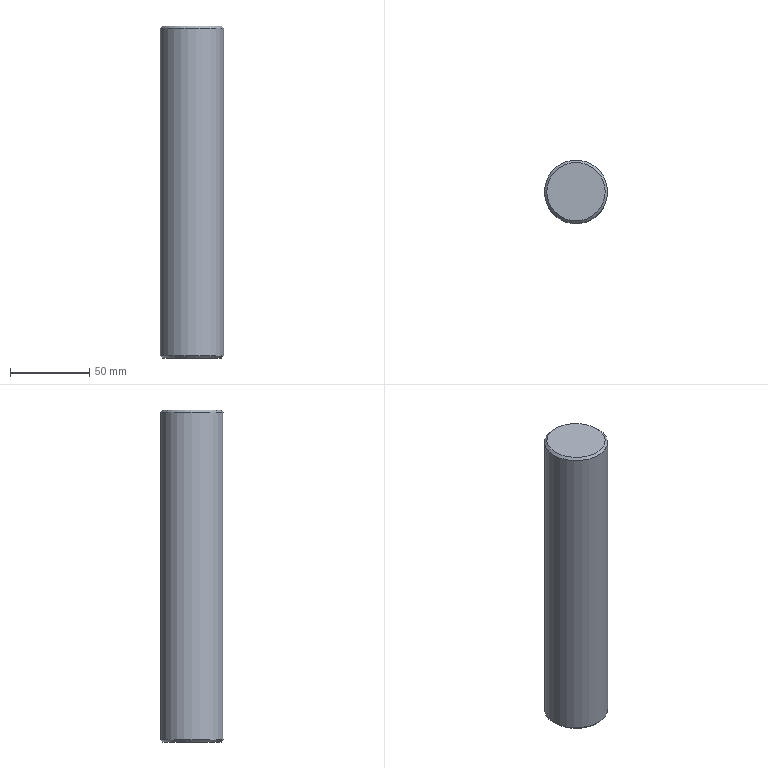Part | STEP file | 车灯-后视镜_id18_x_t | 1 solid | 9 faces | box 40 x 40 x 210 mm | volume 261823 mm3 | cylinder 3 | plane 3 | cone 3 | commonest cylinder face diameters 8.6 x1 10 x1 40 x1
STEP:
#1=CARTESIAN_POINT('',(35.,50.,-162.));
#2=VERTEX_POINT('',#1);
#3=CARTESIAN_POINT('',(15.,50.,-162.));
#4=DIRECTION('',(0.,0.,-1.));
#5=DIRECTION('',(1.,0.,0.));
#6=AXIS2_PLACEMENT_3D('',#3,#4,#5);
#7=CIRCLE('',#6,20.);
#8=EDGE_CURVE('',#2,#2,#7,.T.);
#9=ORIENTED_EDGE('',*,*,#8,.T.);
#10=EDGE_LOOP('',(#9));
#11=FACE_BOUND('',#10,.T.);
#12=CARTESIAN_POINT('',(-5.,50.,-369.));
#13=VERTEX_POINT('',#12);
#14=CARTESIAN_POINT('',(15.,50.,-369.));
#15=DIRECTION('',(0.,0.,1.));
#16=DIRECTION('',(-1.,0.,0.));
#17=AXIS2_PLACEMENT_3D('',#14,#15,#16);
#18=CIRCLE('',#17,20.);
#19=EDGE_CURVE('',#13,#13,#18,.T.);
#20=ORIENTED_EDGE('',*,*,#19,.T.);
#21=EDGE_LOOP('',(#20));
#22=FACE_BOUND('',#21,.T.);
#23=CARTESIAN_POINT('',(15.,50.,-330.5));
#24=DIRECTION('',(0.,0.,1.));
#25=DIRECTION('',(-1.,0.,0.));
#26=AXIS2_PLACEMENT_3D('',#23,#24,#25);
#27=CYLINDRICAL_SURFACE('',#26,20.);
#28=ADVANCED_FACE('',(#11,#22),#27,.T.);
#29=CARTESIAN_POINT('',(33.5,50.,-160.5));
#30=VERTEX_POINT('',#29);
#31=CARTESIAN_POINT('',(15.,50.,-160.5));
#32=DIRECTION('',(0.,0.,1.));
#33=DIRECTION('',(1.,0.,0.));
#34=AXIS2_PLACEMENT_3D('',#31,#32,#33);
#35=CIRCLE('',#34,18.5);
#36=EDGE_CURVE('',#30,#30,#35,.T.);
#37=ORIENTED_EDGE('',*,*,#36,.T.);
#38=EDGE_LOOP('',(#37));
#39=FACE_OUTER_BOUND('',#38,.T.);
#40=CARTESIAN_POINT('',(15.,50.,-160.5));
#41=DIRECTION('',(0.,0.,1.));
#42=DIRECTION('',(-1.,0.,0.));
#43=AXIS2_PLACEMENT_3D('',#40,#41,#42);
#44=PLANE('',#43);
#45=ADVANCED_FACE('',(#39),#44,.T.);
#46=CARTESIAN_POINT('',(-3.5,50.,-370.5));
#47=VERTEX_POINT('',#46);
#48=CARTESIAN_POINT('',(15.,50.,-370.5));
#49=DIRECTION('',(0.,0.,-1.));
#50=DIRECTION('',(-1.,0.,0.));
#51=AXIS2_PLACEMENT_3D('',#48,#49,#50);
#52=CIRCLE('',#51,18.5);
#53=EDGE_CURVE('',#47,#47,#52,.T.);
#54=ORIENTED_EDGE('',*,*,#53,.T.);
#55=EDGE_LOOP('',(#54));
#56=FACE_BOUND('',#55,.T.);
#57=CARTESIAN_POINT('',(10.,50.,-370.5));
#58=VERTEX_POINT('',#57);
#59=CARTESIAN_POINT('',(15.,50.,-370.5));
#60=DIRECTION('',(0.,0.,-1.));
#61=DIRECTION('',(-1.,0.,0.));
#62=AXIS2_PLACEMENT_3D('',#59,#60,#61);
#63=CIRCLE('',#62,5.);
#64=EDGE_CURVE('',#58,#58,#63,.T.);
#65=ORIENTED_EDGE('',*,*,#64,.F.);
#66=EDGE_LOOP('',(#65));
#67=FACE_BOUND('',#66,.T.);
#68=CARTESIAN_POINT('',(15.,50.,-370.5));
#69=DIRECTION('',(0.,0.,-1.));
#70=DIRECTION('',(1.,0.,0.));
#71=AXIS2_PLACEMENT_3D('',#68,#69,#70);
#72=PLANE('',#71);
#73=ADVANCED_FACE('',(#56,#67),#72,.T.);
#74=CARTESIAN_POINT('',(19.3,50.,-347.5));
#75=VERTEX_POINT('',#74);
#76=CARTESIAN_POINT('',(15.,50.,-347.5));
#77=DIRECTION('',(0.,0.,1.));
#78=DIRECTION('',(1.,0.,0.));
#79=AXIS2_PLACEMENT_3D('',#76,#77,#78);
#80=CIRCLE('',#79,4.3);
#81=EDGE_CURVE('',#75,#75,#80,.T.);
#82=ORIENTED_EDGE('',*,*,#81,.T.);
#83=EDGE_LOOP('',(#82));
#84=FACE_BOUND('',#83,.T.);
#85=CARTESIAN_POINT('',(10.7,50.,-350.5));
#86=VERTEX_POINT('',#85);
#87=CARTESIAN_POINT('',(15.,50.,-350.5));
#88=DIRECTION('',(0.,0.,1.));
#89=DIRECTION('',(-1.,0.,0.));
#90=AXIS2_PLACEMENT_3D('',#87,#88,#89);
#91=CIRCLE('',#90,4.3);
#92=EDGE_CURVE('',#86,#86,#91,.T.);
#93=ORIENTED_EDGE('',*,*,#92,.F.);
#94=EDGE_LOOP('',(#93));
#95=FACE_BOUND('',#94,.T.);
#96=CARTESIAN_POINT('',(15.,50.,-350.5));
#97=DIRECTION('',(0.,0.,1.));
#98=DIRECTION('',(-1.,0.,0.));
#99=AXIS2_PLACEMENT_3D('',#96,#97,#98);
#100=CYLINDRICAL_SURFACE('',#99,4.3);
#101=ADVANCED_FACE('',(#84,#95),#100,.F.);
#102=ORIENTED_EDGE('',*,*,#81,.F.);
#103=EDGE_LOOP('',(#102));
#104=FACE_BOUND('',#103,.T.);
#105=CARTESIAN_POINT('',(15.,50.,-344.916));
#106=VERTEX_POINT('',#105);
#107=VERTEX_LOOP('',#106);
#108=FACE_BOUND('',#107,.T.);
#109=CARTESIAN_POINT('',(15.,50.,-344.916));
#110=DIRECTION('',(0.,0.,-1.));
#111=DIRECTION('',(1.,0.,0.));
#112=AXIS2_PLACEMENT_3D('',#109,#110,#111);
#113=CONICAL_SURFACE('',#112,0.,59.);
#114=ADVANCED_FACE('',(#104,#108),#113,.F.);
#115=ORIENTED_EDGE('',*,*,#92,.T.);
#116=EDGE_LOOP('',(#115));
#117=FACE_BOUND('',#116,.T.);
#118=CARTESIAN_POINT('',(20.,50.,-350.5));
#119=VERTEX_POINT('',#118);
#120=CARTESIAN_POINT('',(15.,50.,-350.5));
#121=DIRECTION('',(0.,0.,1.));
#122=DIRECTION('',(1.,0.,0.));
#123=AXIS2_PLACEMENT_3D('',#120,#121,#122);
#124=CIRCLE('',#123,5.);
#125=EDGE_CURVE('',#119,#119,#124,.T.);
#126=ORIENTED_EDGE('',*,*,#125,.F.);
#127=EDGE_LOOP('',(#126));
#128=FACE_BOUND('',#127,.T.);
#129=CARTESIAN_POINT('',(15.,50.,-350.5));
#130=DIRECTION('',(0.,0.,1.));
#131=DIRECTION('',(-1.,0.,0.));
#132=AXIS2_PLACEMENT_3D('',#129,#130,#131);
#133=PLANE('',#132);
#134=ADVANCED_FACE('',(#117,#128),#133,.F.);
#135=ORIENTED_EDGE('',*,*,#125,.T.);
#136=EDGE_LOOP('',(#135));
#137=FACE_BOUND('',#136,.T.);
#138=ORIENTED_EDGE('',*,*,#64,.T.);
#139=EDGE_LOOP('',(#138));
#140=FACE_BOUND('',#139,.T.);
#141=CARTESIAN_POINT('',(15.,50.,-370.5));
#142=DIRECTION('',(0.,0.,1.));
#143=DIRECTION('',(-1.,0.,0.));
#144=AXIS2_PLACEMENT_3D('',#141,#142,#143);
#145=CYLINDRICAL_SURFACE('',#144,5.);
#146=ADVANCED_FACE('',(#137,#140),#145,.F.);
#147=ORIENTED_EDGE('',*,*,#8,.F.);
#148=EDGE_LOOP('',(#147));
#149=FACE_BOUND('',#148,.T.);
#150=ORIENTED_EDGE('',*,*,#36,.F.);
#151=EDGE_LOOP('',(#150));
#152=FACE_BOUND('',#151,.T.);
#153=CARTESIAN_POINT('',(15.,50.,-160.5));
#154=DIRECTION('',(0.,0.,-1.));
#155=DIRECTION('',(-1.,0.,0.));
#156=AXIS2_PLACEMENT_3D('',#153,#154,#155);
#157=CONICAL_SURFACE('',#156,18.5,45.);
#158=ADVANCED_FACE('',(#149,#152),#157,.T.);
#159=ORIENTED_EDGE('',*,*,#53,.F.);
#160=EDGE_LOOP('',(#159));
#161=FACE_BOUND('',#160,.T.);
#162=ORIENTED_EDGE('',*,*,#19,.F.);
#163=EDGE_LOOP('',(#162));
#164=FACE_BOUND('',#163,.T.);
#165=CARTESIAN_POINT('',(15.,50.,-369.));
#166=DIRECTION('',(0.,0.,1.));
#167=DIRECTION('',(1.,0.,0.));
#168=AXIS2_PLACEMENT_3D('',#165,#166,#167);
#169=CONICAL_SURFACE('',#168,20.,45.);
#170=ADVANCED_FACE('',(#161,#164),#169,.T.);
#171=CLOSED_SHELL('',(#28,#45,#73,#101,#114,#134,#146,#158,#170));
#172=MANIFOLD_SOLID_BREP('',#171);
#173=(LENGTH_UNIT()NAMED_UNIT(*)SI_UNIT(.MILLI.,.METRE.));
#174=UNCERTAINTY_MEASURE_WITH_UNIT(LENGTH_MEASURE(0.00002),#173,'','');
#175=(NAMED_UNIT(*)PLANE_ANGLE_UNIT()SI_UNIT($,.RADIAN.));
#176=PLANE_ANGLE_MEASURE_WITH_UNIT(PLANE_ANGLE_MEASURE(0.01745),#175);
#177=DIMENSIONAL_EXPONENTS(0.,0.,0.,0.,0.,0.,0.);
#178=(CONVERSION_BASED_UNIT('DEGREE',#176)NAMED_UNIT(#177)PLANE_ANGLE_UNIT());
#179=(NAMED_UNIT(*)SI_UNIT($,.STERADIAN.)SOLID_ANGLE_UNIT());
#180=(GEOMETRIC_REPRESENTATION_CONTEXT(3)GLOBAL_UNCERTAINTY_ASSIGNED_CONTEXT((#174))GLOBAL_UNIT_ASSIGNED_CONTEXT((#173,#178,#179))REPRESENTATION_CONTEXT('',''));
#181=ADVANCED_BREP_SHAPE_REPRESENTATION('',(#172),#180);